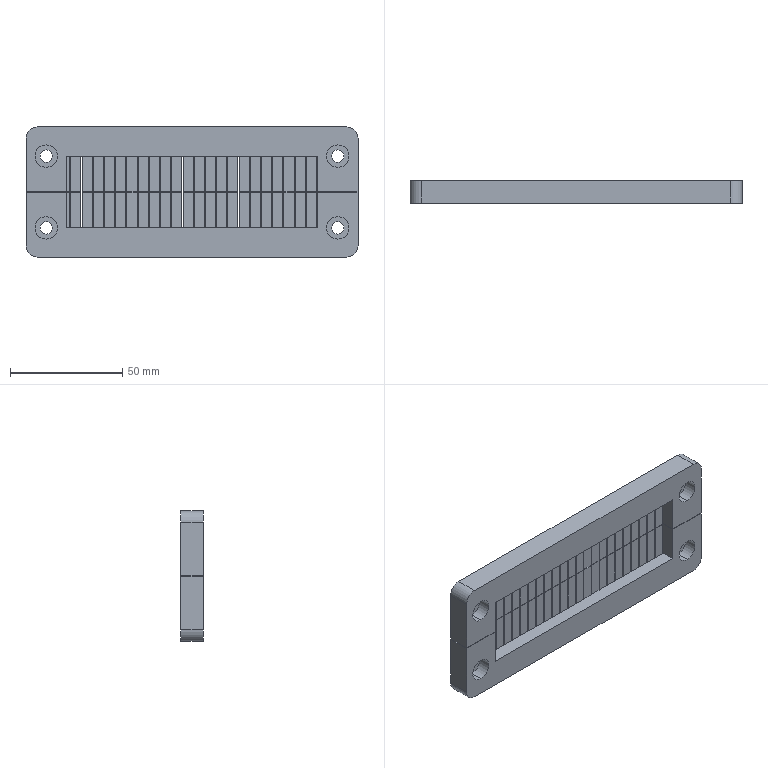Part | STEP file | Cabinet brush KEL-BES-S24 | 2 solids | 224 faces | box 148 x 10 x 58 mm | volume 60298 mm3 | plane 204 | cylinder 20 | commonest cylinder face diameters 10 x12 5.5 x8